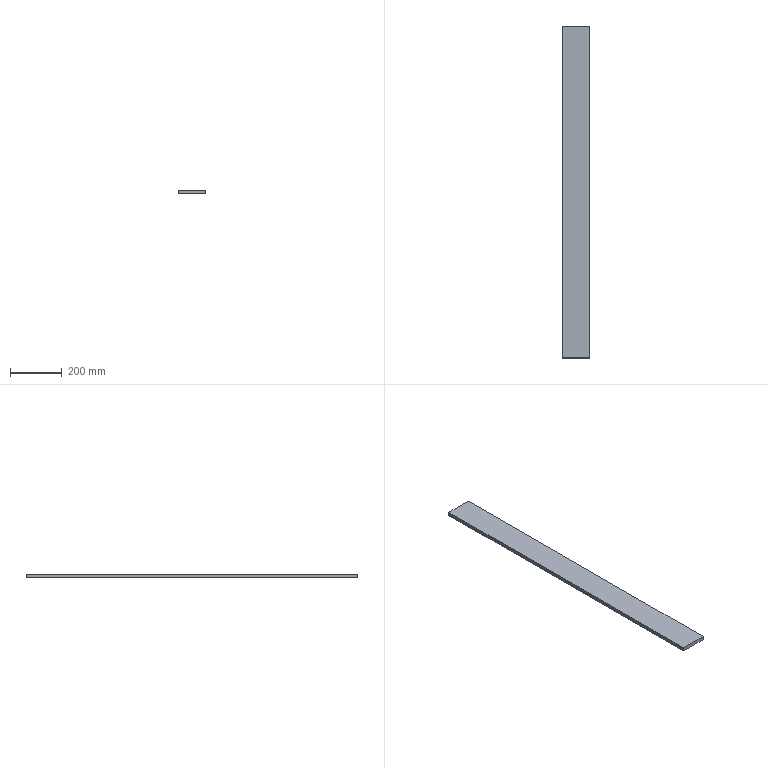Part | STEP file | Part 17 PN_0001_ASM 2 | 1 solid | 6 faces | box 106.46 x 1282 x 15 mm | volume 2047522 mm3 | plane 6
STEP:
#1=CARTESIAN_POINT('',(-171.087,-716.575,0.));
#2=VERTEX_POINT('',#1);
#3=CARTESIAN_POINT('',(-171.087,565.609,0.));
#4=VERTEX_POINT('',#3);
#5=CARTESIAN_POINT('',(-171.087,565.609,0.));
#6=DIRECTION('',(0.,1.,0.));
#7=VECTOR('',#6,1000.);
#8=LINE('',#5,#7);
#9=EDGE_CURVE('',#2,#4,#8,.T.);
#10=ORIENTED_EDGE('',*,*,#9,.T.);
#11=CARTESIAN_POINT('',(-171.087,565.609,15.));
#12=VERTEX_POINT('',#11);
#13=CARTESIAN_POINT('',(-171.087,565.609,15.));
#14=DIRECTION('',(0.,0.,-1.));
#15=VECTOR('',#14,1000.);
#16=LINE('',#13,#15);
#17=EDGE_CURVE('',#12,#4,#16,.T.);
#18=ORIENTED_EDGE('',*,*,#17,.F.);
#19=CARTESIAN_POINT('',(-171.087,-716.575,15.));
#20=VERTEX_POINT('',#19);
#21=CARTESIAN_POINT('',(-171.087,565.609,15.));
#22=DIRECTION('',(0.,1.,0.));
#23=VECTOR('',#22,1000.);
#24=LINE('',#21,#23);
#25=EDGE_CURVE('',#20,#12,#24,.T.);
#26=ORIENTED_EDGE('',*,*,#25,.F.);
#27=CARTESIAN_POINT('',(-171.087,-716.575,15.));
#28=DIRECTION('',(0.,0.,-1.));
#29=VECTOR('',#28,1000.);
#30=LINE('',#27,#29);
#31=EDGE_CURVE('',#20,#2,#30,.T.);
#32=ORIENTED_EDGE('',*,*,#31,.T.);
#33=EDGE_LOOP('',(#10,#18,#26,#32));
#34=FACE_OUTER_BOUND('',#33,.T.);
#35=CARTESIAN_POINT('',(-171.087,565.609,15.));
#36=DIRECTION('',(-1.,0.,0.));
#37=DIRECTION('',(0.,0.,1.));
#38=AXIS2_PLACEMENT_3D('',#35,#36,#37);
#39=PLANE('',#38);
#40=ADVANCED_FACE('',(#34),#39,.F.);
#41=CARTESIAN_POINT('',(-277.547,565.609,0.));
#42=VERTEX_POINT('',#41);
#43=CARTESIAN_POINT('',(-171.087,565.609,0.));
#44=DIRECTION('',(-1.,0.,0.));
#45=VECTOR('',#44,1000.);
#46=LINE('',#43,#45);
#47=EDGE_CURVE('',#4,#42,#46,.T.);
#48=ORIENTED_EDGE('',*,*,#47,.T.);
#49=CARTESIAN_POINT('',(-277.547,565.609,15.));
#50=VERTEX_POINT('',#49);
#51=CARTESIAN_POINT('',(-277.547,565.609,15.));
#52=DIRECTION('',(0.,0.,-1.));
#53=VECTOR('',#52,1000.);
#54=LINE('',#51,#53);
#55=EDGE_CURVE('',#50,#42,#54,.T.);
#56=ORIENTED_EDGE('',*,*,#55,.F.);
#57=CARTESIAN_POINT('',(-171.087,565.609,15.));
#58=DIRECTION('',(-1.,0.,0.));
#59=VECTOR('',#58,1000.);
#60=LINE('',#57,#59);
#61=EDGE_CURVE('',#12,#50,#60,.T.);
#62=ORIENTED_EDGE('',*,*,#61,.F.);
#63=ORIENTED_EDGE('',*,*,#17,.T.);
#64=EDGE_LOOP('',(#48,#56,#62,#63));
#65=FACE_OUTER_BOUND('',#64,.T.);
#66=CARTESIAN_POINT('',(-171.087,565.609,15.));
#67=DIRECTION('',(0.,-1.,0.));
#68=DIRECTION('',(0.,0.,-1.));
#69=AXIS2_PLACEMENT_3D('',#66,#67,#68);
#70=PLANE('',#69);
#71=ADVANCED_FACE('',(#65),#70,.F.);
#72=CARTESIAN_POINT('',(-277.547,-716.575,0.));
#73=VERTEX_POINT('',#72);
#74=CARTESIAN_POINT('',(-277.547,565.609,0.));
#75=DIRECTION('',(0.,-1.,0.));
#76=VECTOR('',#75,1000.);
#77=LINE('',#74,#76);
#78=EDGE_CURVE('',#42,#73,#77,.T.);
#79=ORIENTED_EDGE('',*,*,#78,.T.);
#80=CARTESIAN_POINT('',(-277.547,-716.575,15.));
#81=VERTEX_POINT('',#80);
#82=CARTESIAN_POINT('',(-277.547,-716.575,15.));
#83=DIRECTION('',(0.,0.,-1.));
#84=VECTOR('',#83,1000.);
#85=LINE('',#82,#84);
#86=EDGE_CURVE('',#81,#73,#85,.T.);
#87=ORIENTED_EDGE('',*,*,#86,.F.);
#88=CARTESIAN_POINT('',(-277.547,565.609,15.));
#89=DIRECTION('',(0.,-1.,0.));
#90=VECTOR('',#89,1000.);
#91=LINE('',#88,#90);
#92=EDGE_CURVE('',#50,#81,#91,.T.);
#93=ORIENTED_EDGE('',*,*,#92,.F.);
#94=ORIENTED_EDGE('',*,*,#55,.T.);
#95=EDGE_LOOP('',(#79,#87,#93,#94));
#96=FACE_OUTER_BOUND('',#95,.T.);
#97=CARTESIAN_POINT('',(-277.547,565.609,15.));
#98=DIRECTION('',(1.,0.,0.));
#99=DIRECTION('',(0.,0.,-1.));
#100=AXIS2_PLACEMENT_3D('',#97,#98,#99);
#101=PLANE('',#100);
#102=ADVANCED_FACE('',(#96),#101,.F.);
#103=CARTESIAN_POINT('',(-171.087,-716.575,0.));
#104=DIRECTION('',(1.,0.,0.));
#105=VECTOR('',#104,1000.);
#106=LINE('',#103,#105);
#107=EDGE_CURVE('',#73,#2,#106,.T.);
#108=ORIENTED_EDGE('',*,*,#107,.T.);
#109=ORIENTED_EDGE('',*,*,#31,.F.);
#110=CARTESIAN_POINT('',(-171.087,-716.575,15.));
#111=DIRECTION('',(1.,0.,0.));
#112=VECTOR('',#111,1000.);
#113=LINE('',#110,#112);
#114=EDGE_CURVE('',#81,#20,#113,.T.);
#115=ORIENTED_EDGE('',*,*,#114,.F.);
#116=ORIENTED_EDGE('',*,*,#86,.T.);
#117=EDGE_LOOP('',(#108,#109,#115,#116));
#118=FACE_OUTER_BOUND('',#117,.T.);
#119=CARTESIAN_POINT('',(-171.087,-716.575,15.));
#120=DIRECTION('',(0.,1.,0.));
#121=DIRECTION('',(0.,0.,1.));
#122=AXIS2_PLACEMENT_3D('',#119,#120,#121);
#123=PLANE('',#122);
#124=ADVANCED_FACE('',(#118),#123,.F.);
#125=ORIENTED_EDGE('',*,*,#25,.T.);
#126=ORIENTED_EDGE('',*,*,#61,.T.);
#127=ORIENTED_EDGE('',*,*,#92,.T.);
#128=ORIENTED_EDGE('',*,*,#114,.T.);
#129=EDGE_LOOP('',(#125,#126,#127,#128));
#130=FACE_OUTER_BOUND('',#129,.T.);
#131=CARTESIAN_POINT('',(-171.087,-716.575,15.));
#132=DIRECTION('',(0.,0.,-1.));
#133=DIRECTION('',(-1.,0.,0.));
#134=AXIS2_PLACEMENT_3D('',#131,#132,#133);
#135=PLANE('',#134);
#136=ADVANCED_FACE('',(#130),#135,.F.);
#137=ORIENTED_EDGE('',*,*,#9,.F.);
#138=ORIENTED_EDGE('',*,*,#107,.F.);
#139=ORIENTED_EDGE('',*,*,#78,.F.);
#140=ORIENTED_EDGE('',*,*,#47,.F.);
#141=EDGE_LOOP('',(#137,#138,#139,#140));
#142=FACE_OUTER_BOUND('',#141,.T.);
#143=CARTESIAN_POINT('',(-171.087,-716.575,0.));
#144=DIRECTION('',(0.,0.,-1.));
#145=DIRECTION('',(-1.,0.,0.));
#146=AXIS2_PLACEMENT_3D('',#143,#144,#145);
#147=PLANE('',#146);
#148=ADVANCED_FACE('',(#142),#147,.T.);
#149=CLOSED_SHELL('',(#40,#71,#102,#124,#136,#148));
#150=MANIFOLD_SOLID_BREP('',#149);
#151=CARTESIAN_POINT('',(0.,0.,0.));
#152=DIRECTION('',(0.,0.,1.));
#153=DIRECTION('',(1.,0.,0.));
#154=AXIS2_PLACEMENT_3D('',#151,#152,#153);
#155=(LENGTH_UNIT()NAMED_UNIT(*)SI_UNIT(.MILLI.,.METRE.));
#156=UNCERTAINTY_MEASURE_WITH_UNIT(LENGTH_MEASURE(0.00001),#155,'','');
#157=(NAMED_UNIT(*)PLANE_ANGLE_UNIT()SI_UNIT($,.RADIAN.));
#158=(NAMED_UNIT(*)SI_UNIT($,.STERADIAN.)SOLID_ANGLE_UNIT());
#159=(GEOMETRIC_REPRESENTATION_CONTEXT(3)GLOBAL_UNCERTAINTY_ASSIGNED_CONTEXT((#156))GLOBAL_UNIT_ASSIGNED_CONTEXT((#155,#157,#158))REPRESENTATION_CONTEXT('',''));
#160=ADVANCED_BREP_SHAPE_REPRESENTATION('',(#150,#154),#159);